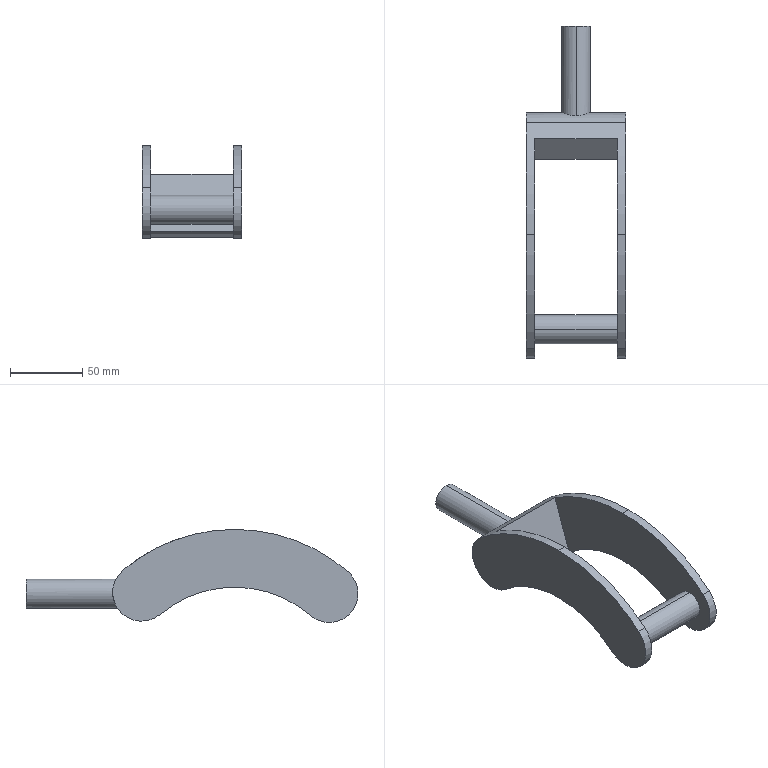Part | SolidWorks | features ICE 4, Extrusion 1 | 1 solid | 20 faces | box 69 x 230 x 64.48 mm | volume 170507 mm3 | cylinder 14 | plane 6 | commonest cylinder face diameters 20 x4 160 x4 40 x3 240 x3
STEP:
#1=CARTESIAN_POINT('',(0.,210.,10.));
#2=VERTEX_POINT('',#1);
#3=CARTESIAN_POINT('',(0.,210.,-10.));
#4=VERTEX_POINT('',#3);
#5=CARTESIAN_POINT('',(0.,210.,0.));
#6=DIRECTION('',(0.,1.,0.));
#7=DIRECTION('',(0.,0.,1.));
#8=AXIS2_PLACEMENT_3D('',#5,#6,#7);
#9=CIRCLE('',#8,10.);
#10=EDGE_CURVE('',#2,#4,#9,.T.);
#11=ORIENTED_EDGE('',*,*,#10,.F.);
#12=CARTESIAN_POINT('',(0.,147.831,10.));
#13=VERTEX_POINT('',#12);
#14=CARTESIAN_POINT('',(0.,210.,10.));
#15=DIRECTION('',(0.,-1.,0.));
#16=VECTOR('',#15,1000.);
#17=LINE('',#14,#16);
#18=EDGE_CURVE('',#2,#13,#17,.T.);
#19=ORIENTED_EDGE('',*,*,#18,.T.);
#20=CARTESIAN_POINT('',(0.,146.742,-10.));
#21=VERTEX_POINT('',#20);
#22=CARTESIAN_POINT('',(0.,147.831,10.));
#23=CARTESIAN_POINT('',(0.6634,147.831,10.));
#24=CARTESIAN_POINT('',(1.339,147.866,9.932));
#25=CARTESIAN_POINT('',(2.636,147.996,9.669));
#26=CARTESIAN_POINT('',(3.265,148.09,9.475));
#27=CARTESIAN_POINT('',(4.486,148.323,8.962));
#28=CARTESIAN_POINT('',(5.059,148.458,8.651));
#29=CARTESIAN_POINT('',(5.866,148.674,8.105));
#30=CARTESIAN_POINT('',(6.126,148.748,7.911));
#31=CARTESIAN_POINT('',(6.63,148.897,7.494));
#32=CARTESIAN_POINT('',(6.871,148.973,7.273));
#33=CARTESIAN_POINT('',(7.557,149.194,6.582));
#34=CARTESIAN_POINT('',(7.966,149.336,6.08));
#35=CARTESIAN_POINT('',(8.509,149.529,5.263));
#36=CARTESIAN_POINT('',(8.679,149.591,4.978));
#37=CARTESIAN_POINT('',(8.988,149.702,4.396));
#38=CARTESIAN_POINT('',(9.128,149.752,4.098));
#39=CARTESIAN_POINT('',(9.501,149.883,3.188));
#40=CARTESIAN_POINT('',(9.691,149.946,2.556));
#41=CARTESIAN_POINT('',(9.882,149.993,1.568));
#42=CARTESIAN_POINT('',(9.929,150.001,1.235));
#43=CARTESIAN_POINT('',(9.989,149.999,0.5732));
#44=CARTESIAN_POINT('',(10.016,149.982,-0.08898));
#45=CARTESIAN_POINT('',(9.977,149.931,-0.7512));
#46=CARTESIAN_POINT('',(9.905,149.864,-1.413));
#47=CARTESIAN_POINT('',(9.852,149.822,-1.744));
#48=CARTESIAN_POINT('',(9.648,149.674,-2.712));
#49=CARTESIAN_POINT('',(9.45,149.548,-3.334));
#50=CARTESIAN_POINT('',(9.065,149.321,-4.234));
#51=CARTESIAN_POINT('',(8.922,149.24,-4.528));
#52=CARTESIAN_POINT('',(8.611,149.07,-5.094));
#53=CARTESIAN_POINT('',(8.444,148.981,-5.367));
#54=CARTESIAN_POINT('',(8.084,148.798,-5.895));
#55=CARTESIAN_POINT('',(7.892,148.703,-6.15));
#56=CARTESIAN_POINT('',(7.483,148.509,-6.641));
#57=CARTESIAN_POINT('',(7.265,148.41,-6.879));
#58=CARTESIAN_POINT('',(6.585,148.113,-7.553));
#59=CARTESIAN_POINT('',(6.094,147.918,-7.954));
#60=CARTESIAN_POINT('',(5.299,147.64,-8.487));
#61=CARTESIAN_POINT('',(5.023,147.55,-8.653));
#62=CARTESIAN_POINT('',(4.452,147.378,-8.96));
#63=CARTESIAN_POINT('',(4.158,147.297,-9.1));
#64=CARTESIAN_POINT('',(3.262,147.076,-9.475));
#65=CARTESIAN_POINT('',(2.642,146.956,-9.667));
#66=CARTESIAN_POINT('',(1.349,146.788,-9.93));
#67=CARTESIAN_POINT('',(0.673,146.742,-10.));
#68=CARTESIAN_POINT('',(0.,146.742,-10.));
#69=B_SPLINE_CURVE_WITH_KNOTS('',3,(#22,#23,#24,#25,#26,#27,#28,#29,#30,#31,#32,#33,#34,#35,#36,#37,#38,#39,#40,#41,#42,#43,#44,#45,#46,#47,#48,#49,#50,#51,#52,#53,#54,#55,#56,#57,#58,#59,#60,#61,#62,#63,#64,#65,#66,#67,#68),.UNSPECIFIED.,.F.,.F.,(4,2,2,2,2,2,2,2,2,2,2,1,2,2,2,2,2,2,2,2,2,2,2,4),(0.03183,0.03381,0.0358,0.03778,0.03878,0.03977,0.04176,0.04275,0.04374,0.04573,0.04672,0.04772,0.04871,0.0497,0.05169,0.05268,0.05367,0.05467,0.05566,0.05765,0.05864,0.05963,0.06162,0.06361),.UNSPECIFIED.);
#70=EDGE_CURVE('',#13,#21,#69,.T.);
#71=ORIENTED_EDGE('',*,*,#70,.T.);
#72=CARTESIAN_POINT('',(0.,210.,-10.));
#73=DIRECTION('',(0.,-1.,0.));
#74=VECTOR('',#73,1000.);
#75=LINE('',#72,#74);
#76=EDGE_CURVE('',#4,#21,#75,.T.);
#77=ORIENTED_EDGE('',*,*,#76,.F.);
#78=EDGE_LOOP('',(#11,#19,#71,#77));
#79=FACE_OUTER_BOUND('',#78,.T.);
#80=CARTESIAN_POINT('',(0.,210.,0.));
#81=DIRECTION('',(0.,-1.,0.));
#82=DIRECTION('',(0.,0.,-1.));
#83=AXIS2_PLACEMENT_3D('',#80,#81,#82);
#84=CYLINDRICAL_SURFACE('',#83,10.);
#85=ADVANCED_FACE('',(#79),#84,.T.);
#86=CARTESIAN_POINT('',(28.5,0.,10.));
#87=VERTEX_POINT('',#86);
#88=CARTESIAN_POINT('',(28.5,0.,-10.));
#89=VERTEX_POINT('',#88);
#90=CARTESIAN_POINT('',(28.5,0.,0.));
#91=DIRECTION('',(-1.,0.,0.));
#92=DIRECTION('',(0.,0.,-1.));
#93=AXIS2_PLACEMENT_3D('',#90,#91,#92);
#94=CIRCLE('',#93,10.);
#95=EDGE_CURVE('',#87,#89,#94,.T.);
#96=ORIENTED_EDGE('',*,*,#95,.T.);
#97=CARTESIAN_POINT('',(-28.5,0.,-10.));
#98=VERTEX_POINT('',#97);
#99=CARTESIAN_POINT('',(29.,0.,-10.));
#100=DIRECTION('',(-1.,0.,0.));
#101=VECTOR('',#100,1000.);
#102=LINE('',#99,#101);
#103=EDGE_CURVE('',#89,#98,#102,.T.);
#104=ORIENTED_EDGE('',*,*,#103,.T.);
#105=CARTESIAN_POINT('',(-28.5,0.,10.));
#106=VERTEX_POINT('',#105);
#107=CARTESIAN_POINT('',(-28.5,0.,0.));
#108=DIRECTION('',(-1.,0.,0.));
#109=DIRECTION('',(0.,0.,-1.));
#110=AXIS2_PLACEMENT_3D('',#107,#108,#109);
#111=CIRCLE('',#110,10.);
#112=EDGE_CURVE('',#106,#98,#111,.T.);
#113=ORIENTED_EDGE('',*,*,#112,.F.);
#114=CARTESIAN_POINT('',(29.,0.,10.));
#115=DIRECTION('',(-1.,0.,0.));
#116=VECTOR('',#115,1000.);
#117=LINE('',#114,#116);
#118=EDGE_CURVE('',#87,#106,#117,.T.);
#119=ORIENTED_EDGE('',*,*,#118,.F.);
#120=EDGE_LOOP('',(#96,#104,#113,#119));
#121=FACE_OUTER_BOUND('',#120,.T.);
#122=CARTESIAN_POINT('',(29.,0.,0.));
#123=DIRECTION('',(-1.,0.,0.));
#124=DIRECTION('',(0.,0.,1.));
#125=AXIS2_PLACEMENT_3D('',#122,#123,#124);
#126=CYLINDRICAL_SURFACE('',#125,10.);
#127=ADVANCED_FACE('',(#121),#126,.T.);
#128=CARTESIAN_POINT('',(-28.5,65.55,4.48));
#129=VERTEX_POINT('',#128);
#130=CARTESIAN_POINT('',(-28.5,117.11,-14.351));
#131=VERTEX_POINT('',#130);
#132=CARTESIAN_POINT('',(-28.5,65.55,-75.52));
#133=DIRECTION('',(-1.,0.,0.));
#134=DIRECTION('',(0.,0.,-1.));
#135=AXIS2_PLACEMENT_3D('',#132,#133,#134);
#136=CIRCLE('',#135,80.);
#137=EDGE_CURVE('',#129,#131,#136,.T.);
#138=ORIENTED_EDGE('',*,*,#137,.F.);
#139=CARTESIAN_POINT('',(-34.5,65.55,4.48));
#140=VERTEX_POINT('',#139);
#141=CARTESIAN_POINT('',(34.5,65.55,4.48));
#142=DIRECTION('',(-1.,0.,0.));
#143=VECTOR('',#142,1000.);
#144=LINE('',#141,#143);
#145=EDGE_CURVE('',#129,#140,#144,.T.);
#146=ORIENTED_EDGE('',*,*,#145,.T.);
#147=CARTESIAN_POINT('',(-34.5,117.11,-14.351));
#148=VERTEX_POINT('',#147);
#149=CARTESIAN_POINT('',(-34.5,65.55,-75.52));
#150=DIRECTION('',(-1.,0.,0.));
#151=DIRECTION('',(0.,0.,-1.));
#152=AXIS2_PLACEMENT_3D('',#149,#150,#151);
#153=CIRCLE('',#152,80.);
#154=EDGE_CURVE('',#140,#148,#153,.T.);
#155=ORIENTED_EDGE('',*,*,#154,.T.);
#156=CARTESIAN_POINT('',(34.5,117.11,-14.351));
#157=DIRECTION('',(-1.,0.,0.));
#158=VECTOR('',#157,1000.);
#159=LINE('',#156,#158);
#160=EDGE_CURVE('',#131,#148,#159,.T.);
#161=ORIENTED_EDGE('',*,*,#160,.F.);
#162=EDGE_LOOP('',(#138,#146,#155,#161));
#163=FACE_OUTER_BOUND('',#162,.T.);
#164=CARTESIAN_POINT('',(34.5,65.55,-75.52));
#165=DIRECTION('',(-1.,0.,0.));
#166=DIRECTION('',(0.,0.,1.));
#167=AXIS2_PLACEMENT_3D('',#164,#165,#166);
#168=CYLINDRICAL_SURFACE('',#167,80.);
#169=ADVANCED_FACE('',(#163),#168,.F.);
#170=CARTESIAN_POINT('',(34.5,65.55,4.48));
#171=VERTEX_POINT('',#170);
#172=CARTESIAN_POINT('',(34.5,117.11,-14.351));
#173=VERTEX_POINT('',#172);
#174=CARTESIAN_POINT('',(34.5,65.55,-75.52));
#175=DIRECTION('',(-1.,0.,0.));
#176=DIRECTION('',(0.,0.,-1.));
#177=AXIS2_PLACEMENT_3D('',#174,#175,#176);
#178=CIRCLE('',#177,80.);
#179=EDGE_CURVE('',#171,#173,#178,.T.);
#180=ORIENTED_EDGE('',*,*,#179,.F.);
#181=CARTESIAN_POINT('',(28.5,65.55,4.48));
#182=VERTEX_POINT('',#181);
#183=CARTESIAN_POINT('',(34.5,65.55,4.48));
#184=DIRECTION('',(-1.,0.,0.));
#185=VECTOR('',#184,1000.);
#186=LINE('',#183,#185);
#187=EDGE_CURVE('',#171,#182,#186,.T.);
#188=ORIENTED_EDGE('',*,*,#187,.T.);
#189=CARTESIAN_POINT('',(28.5,117.11,-14.351));
#190=VERTEX_POINT('',#189);
#191=CARTESIAN_POINT('',(28.5,65.55,-75.52));
#192=DIRECTION('',(-1.,0.,0.));
#193=DIRECTION('',(0.,0.,-1.));
#194=AXIS2_PLACEMENT_3D('',#191,#192,#193);
#195=CIRCLE('',#194,80.);
#196=EDGE_CURVE('',#182,#190,#195,.T.);
#197=ORIENTED_EDGE('',*,*,#196,.T.);
#198=CARTESIAN_POINT('',(34.5,117.11,-14.351));
#199=DIRECTION('',(-1.,0.,0.));
#200=VECTOR('',#199,1000.);
#201=LINE('',#198,#200);
#202=EDGE_CURVE('',#173,#190,#201,.T.);
#203=ORIENTED_EDGE('',*,*,#202,.F.);
#204=EDGE_LOOP('',(#180,#188,#197,#203));
#205=FACE_OUTER_BOUND('',#204,.T.);
#206=CARTESIAN_POINT('',(34.5,65.55,-75.52));
#207=DIRECTION('',(-1.,0.,0.));
#208=DIRECTION('',(0.,0.,1.));
#209=AXIS2_PLACEMENT_3D('',#206,#207,#208);
#210=CYLINDRICAL_SURFACE('',#209,80.);
#211=ADVANCED_FACE('',(#205),#210,.F.);
#212=CARTESIAN_POINT('',(34.5,65.55,44.48));
#213=VERTEX_POINT('',#212);
#214=CARTESIAN_POINT('',(34.5,-13.11,15.104));
#215=VERTEX_POINT('',#214);
#216=CARTESIAN_POINT('',(34.5,65.55,-75.52));
#217=DIRECTION('',(1.,0.,0.));
#218=DIRECTION('',(0.,0.,-1.));
#219=AXIS2_PLACEMENT_3D('',#216,#217,#218);
#220=CIRCLE('',#219,120.);
#221=EDGE_CURVE('',#213,#215,#220,.T.);
#222=ORIENTED_EDGE('',*,*,#221,.F.);
#223=CARTESIAN_POINT('',(28.5,65.55,44.48));
#224=VERTEX_POINT('',#223);
#225=CARTESIAN_POINT('',(34.5,65.55,44.48));
#226=DIRECTION('',(-1.,0.,0.));
#227=VECTOR('',#226,1000.);
#228=LINE('',#225,#227);
#229=EDGE_CURVE('',#213,#224,#228,.T.);
#230=ORIENTED_EDGE('',*,*,#229,.T.);
#231=CARTESIAN_POINT('',(28.5,-13.11,15.104));
#232=VERTEX_POINT('',#231);
#233=CARTESIAN_POINT('',(28.5,65.55,-75.52));
#234=DIRECTION('',(1.,0.,0.));
#235=DIRECTION('',(0.,0.,-1.));
#236=AXIS2_PLACEMENT_3D('',#233,#234,#235);
#237=CIRCLE('',#236,120.);
#238=EDGE_CURVE('',#224,#232,#237,.T.);
#239=ORIENTED_EDGE('',*,*,#238,.T.);
#240=CARTESIAN_POINT('',(34.5,-13.11,15.104));
#241=DIRECTION('',(-1.,0.,0.));
#242=VECTOR('',#241,1000.);
#243=LINE('',#240,#242);
#244=EDGE_CURVE('',#215,#232,#243,.T.);
#245=ORIENTED_EDGE('',*,*,#244,.F.);
#246=EDGE_LOOP('',(#222,#230,#239,#245));
#247=FACE_OUTER_BOUND('',#246,.T.);
#248=CARTESIAN_POINT('',(34.5,65.55,-75.52));
#249=DIRECTION('',(-1.,0.,0.));
#250=DIRECTION('',(0.,0.,1.));
#251=AXIS2_PLACEMENT_3D('',#248,#249,#250);
#252=CYLINDRICAL_SURFACE('',#251,120.);
#253=ADVANCED_FACE('',(#247),#252,.T.);
#254=CARTESIAN_POINT('',(-28.5,65.55,44.48));
#255=VERTEX_POINT('',#254);
#256=CARTESIAN_POINT('',(-28.5,-13.11,15.104));
#257=VERTEX_POINT('',#256);
#258=CARTESIAN_POINT('',(-28.5,65.55,-75.52));
#259=DIRECTION('',(1.,0.,0.));
#260=DIRECTION('',(0.,0.,-1.));
#261=AXIS2_PLACEMENT_3D('',#258,#259,#260);
#262=CIRCLE('',#261,120.);
#263=EDGE_CURVE('',#255,#257,#262,.T.);
#264=ORIENTED_EDGE('',*,*,#263,.F.);
#265=CARTESIAN_POINT('',(-34.5,65.55,44.48));
#266=VERTEX_POINT('',#265);
#267=CARTESIAN_POINT('',(34.5,65.55,44.48));
#268=DIRECTION('',(-1.,0.,0.));
#269=VECTOR('',#268,1000.);
#270=LINE('',#267,#269);
#271=EDGE_CURVE('',#255,#266,#270,.T.);
#272=ORIENTED_EDGE('',*,*,#271,.T.);
#273=CARTESIAN_POINT('',(-34.5,-13.11,15.104));
#274=VERTEX_POINT('',#273);
#275=CARTESIAN_POINT('',(-34.5,65.55,-75.52));
#276=DIRECTION('',(1.,0.,0.));
#277=DIRECTION('',(0.,0.,-1.));
#278=AXIS2_PLACEMENT_3D('',#275,#276,#277);
#279=CIRCLE('',#278,120.);
#280=EDGE_CURVE('',#266,#274,#279,.T.);
#281=ORIENTED_EDGE('',*,*,#280,.T.);
#282=CARTESIAN_POINT('',(34.5,-13.11,15.104));
#283=DIRECTION('',(-1.,0.,0.));
#284=VECTOR('',#283,1000.);
#285=LINE('',#282,#284);
#286=EDGE_CURVE('',#257,#274,#285,.T.);
#287=ORIENTED_EDGE('',*,*,#286,.F.);
#288=EDGE_LOOP('',(#264,#272,#281,#287));
#289=FACE_OUTER_BOUND('',#288,.T.);
#290=CARTESIAN_POINT('',(34.5,65.55,-75.52));
#291=DIRECTION('',(-1.,0.,0.));
#292=DIRECTION('',(0.,0.,1.));
#293=AXIS2_PLACEMENT_3D('',#290,#291,#292);
#294=CYLINDRICAL_SURFACE('',#293,120.);
#295=ADVANCED_FACE('',(#289),#294,.T.);
#296=CARTESIAN_POINT('',(28.5,117.742,-14.862));
#297=VERTEX_POINT('',#296);
#298=CARTESIAN_POINT('',(28.5,130.,0.9408));
#299=DIRECTION('',(-1.,0.,0.));
#300=DIRECTION('',(0.,0.,1.));
#301=AXIS2_PLACEMENT_3D('',#298,#299,#300);
#302=CIRCLE('',#301,20.);
#303=EDGE_CURVE('',#297,#190,#302,.T.);
#304=ORIENTED_EDGE('',*,*,#303,.F.);
#305=CARTESIAN_POINT('',(-28.5,117.742,-14.862));
#306=VERTEX_POINT('',#305);
#307=CARTESIAN_POINT('',(34.5,117.742,-14.862));
#308=DIRECTION('',(1.,0.,0.));
#309=VECTOR('',#308,1000.);
#310=LINE('',#307,#309);
#311=EDGE_CURVE('',#306,#297,#310,.T.);
#312=ORIENTED_EDGE('',*,*,#311,.F.);
#313=CARTESIAN_POINT('',(-28.5,130.,0.9408));
#314=DIRECTION('',(1.,0.,0.));
#315=DIRECTION('',(0.,0.,-1.));
#316=AXIS2_PLACEMENT_3D('',#313,#314,#315);
#317=CIRCLE('',#316,20.);
#318=EDGE_CURVE('',#131,#306,#317,.T.);
#319=ORIENTED_EDGE('',*,*,#318,.F.);
#320=ORIENTED_EDGE('',*,*,#160,.T.);
#321=CARTESIAN_POINT('',(-34.5,142.89,16.233));
#322=VERTEX_POINT('',#321);
#323=CARTESIAN_POINT('',(-34.5,130.,0.9408));
#324=DIRECTION('',(1.,0.,0.));
#325=DIRECTION('',(0.,0.,-1.));
#326=AXIS2_PLACEMENT_3D('',#323,#324,#325);
#327=CIRCLE('',#326,20.);
#328=EDGE_CURVE('',#148,#322,#327,.T.);
#329=ORIENTED_EDGE('',*,*,#328,.T.);
#330=CARTESIAN_POINT('',(34.5,142.89,16.233));
#331=VERTEX_POINT('',#330);
#332=CARTESIAN_POINT('',(34.5,142.89,16.233));
#333=DIRECTION('',(-1.,0.,0.));
#334=VECTOR('',#333,1000.);
#335=LINE('',#332,#334);
#336=EDGE_CURVE('',#331,#322,#335,.T.);
#337=ORIENTED_EDGE('',*,*,#336,.F.);
#338=CARTESIAN_POINT('',(34.5,130.,0.9408));
#339=DIRECTION('',(1.,0.,0.));
#340=DIRECTION('',(0.,0.,-1.));
#341=AXIS2_PLACEMENT_3D('',#338,#339,#340);
#342=CIRCLE('',#341,20.);
#343=EDGE_CURVE('',#173,#331,#342,.T.);
#344=ORIENTED_EDGE('',*,*,#343,.F.);
#345=ORIENTED_EDGE('',*,*,#202,.T.);
#346=EDGE_LOOP('',(#304,#312,#319,#320,#329,#337,#344,#345));
#347=FACE_OUTER_BOUND('',#346,.T.);
#348=CARTESIAN_POINT('',(0.,146.742,-10.));
#349=CARTESIAN_POINT('',(-0.674,146.742,-10.));
#350=CARTESIAN_POINT('',(-1.333,146.787,-9.933));
#351=CARTESIAN_POINT('',(-2.625,146.953,-9.672));
#352=CARTESIAN_POINT('',(-3.263,147.076,-9.475));
#353=CARTESIAN_POINT('',(-4.461,147.372,-8.973));
#354=CARTESIAN_POINT('',(-5.027,147.545,-8.669));
#355=CARTESIAN_POINT('',(-6.098,147.919,-7.951));
#356=CARTESIAN_POINT('',(-6.592,148.117,-7.546));
#357=CARTESIAN_POINT('',(-7.268,148.411,-6.876));
#358=CARTESIAN_POINT('',(-7.483,148.509,-6.641));
#359=CARTESIAN_POINT('',(-7.892,148.703,-6.149));
#360=CARTESIAN_POINT('',(-8.087,148.799,-5.891));
#361=CARTESIAN_POINT('',(-8.628,149.076,-5.095));
#362=CARTESIAN_POINT('',(-8.936,149.246,-4.534));
#363=CARTESIAN_POINT('',(-9.318,149.47,-3.644));
#364=CARTESIAN_POINT('',(-9.432,149.54,-3.338));
#365=CARTESIAN_POINT('',(-9.631,149.667,-2.71));
#366=CARTESIAN_POINT('',(-9.716,149.723,-2.39));
#367=CARTESIAN_POINT('',(-9.92,149.87,-1.424));
#368=CARTESIAN_POINT('',(-9.992,149.938,-0.7701));
#369=CARTESIAN_POINT('',(-10.003,149.99,0.2283));
#370=CARTESIAN_POINT('',(-9.99,149.999,0.5662));
#371=CARTESIAN_POINT('',(-9.929,150.001,1.233));
#372=CARTESIAN_POINT('',(-9.883,149.993,1.563));
#373=CARTESIAN_POINT('',(-9.757,149.962,2.214));
#374=CARTESIAN_POINT('',(-9.679,149.939,2.536));
#375=CARTESIAN_POINT('',(-9.489,149.878,3.173));
#376=CARTESIAN_POINT('',(-9.378,149.839,3.489));
#377=CARTESIAN_POINT('',(-8.999,149.706,4.411));
#378=CARTESIAN_POINT('',(-8.691,149.594,4.99));
#379=CARTESIAN_POINT('',(-8.147,149.401,5.808));
#380=CARTESIAN_POINT('',(-7.951,149.332,6.073));
#381=CARTESIAN_POINT('',(-7.537,149.19,6.581));
#382=CARTESIAN_POINT('',(-7.319,149.117,6.822));
#383=CARTESIAN_POINT('',(-6.633,148.896,7.512));
#384=CARTESIAN_POINT('',(-6.133,148.745,7.925));
#385=CARTESIAN_POINT('',(-5.045,148.455,8.659));
#386=CARTESIAN_POINT('',(-4.47,148.32,8.969));
#387=CARTESIAN_POINT('',(-3.567,148.148,9.348));
#388=CARTESIAN_POINT('',(-3.259,148.095,9.46));
#389=CARTESIAN_POINT('',(-2.628,148.002,9.654));
#390=CARTESIAN_POINT('',(-2.303,147.962,9.737));
#391=CARTESIAN_POINT('',(-1.323,147.864,9.934));
#392=CARTESIAN_POINT('',(-0.6644,147.831,10.));
#393=CARTESIAN_POINT('',(0.,147.831,10.));
#394=B_SPLINE_CURVE_WITH_KNOTS('',3,(#348,#349,#350,#351,#352,#353,#354,#355,#356,#357,#358,#359,#360,#361,#362,#363,#364,#365,#366,#367,#368,#369,#370,#371,#372,#373,#374,#375,#376,#377,#378,#379,#380,#381,#382,#383,#384,#385,#386,#387,#388,#389,#390,#391,#392,#393),.UNSPECIFIED.,.F.,.F.,(4,2,2,2,2,2,2,2,2,2,2,2,2,2,2,2,2,2,2,2,2,2,4),(0.,0.001989,0.003978,0.005967,0.007956,0.008951,0.009946,0.01193,0.01293,0.01392,0.01591,0.01691,0.0179,0.0189,0.01989,0.02188,0.02287,0.02387,0.02586,0.02785,0.02884,0.02984,0.03183),.UNSPECIFIED.);
#395=EDGE_CURVE('',#21,#13,#394,.T.);
#396=ORIENTED_EDGE('',*,*,#395,.F.);
#397=ORIENTED_EDGE('',*,*,#70,.F.);
#398=EDGE_LOOP('',(#396,#397));
#399=FACE_BOUND('',#398,.T.);
#400=CARTESIAN_POINT('',(34.5,130.,0.9408));
#401=DIRECTION('',(-1.,0.,0.));
#402=DIRECTION('',(0.,0.,1.));
#403=AXIS2_PLACEMENT_3D('',#400,#401,#402);
#404=CYLINDRICAL_SURFACE('',#403,20.);
#405=ADVANCED_FACE('',(#347,#399),#404,.T.);
#406=ORIENTED_EDGE('',*,*,#229,.F.);
#407=CARTESIAN_POINT('',(34.5,65.55,-75.52));
#408=DIRECTION('',(1.,0.,0.));
#409=DIRECTION('',(0.,0.,-1.));
#410=AXIS2_PLACEMENT_3D('',#407,#408,#409);
#411=CIRCLE('',#410,120.);
#412=EDGE_CURVE('',#331,#213,#411,.T.);
#413=ORIENTED_EDGE('',*,*,#412,.F.);
#414=ORIENTED_EDGE('',*,*,#336,.T.);
#415=CARTESIAN_POINT('',(-34.5,65.55,-75.52));
#416=DIRECTION('',(1.,0.,0.));
#417=DIRECTION('',(0.,0.,-1.));
#418=AXIS2_PLACEMENT_3D('',#415,#416,#417);
#419=CIRCLE('',#418,120.);
#420=EDGE_CURVE('',#322,#266,#419,.T.);
#421=ORIENTED_EDGE('',*,*,#420,.T.);
#422=ORIENTED_EDGE('',*,*,#271,.F.);
#423=CARTESIAN_POINT('',(-28.5,131.974,24.42));
#424=VERTEX_POINT('',#423);
#425=CARTESIAN_POINT('',(-28.5,65.55,-75.52));
#426=DIRECTION('',(1.,0.,0.));
#427=DIRECTION('',(0.,0.,-1.));
#428=AXIS2_PLACEMENT_3D('',#425,#426,#427);
#429=CIRCLE('',#428,120.);
#430=EDGE_CURVE('',#424,#255,#429,.T.);
#431=ORIENTED_EDGE('',*,*,#430,.F.);
#432=CARTESIAN_POINT('',(28.5,131.974,24.42));
#433=VERTEX_POINT('',#432);
#434=CARTESIAN_POINT('',(34.5,131.974,24.42));
#435=DIRECTION('',(-1.,0.,0.));
#436=VECTOR('',#435,1000.);
#437=LINE('',#434,#436);
#438=EDGE_CURVE('',#433,#424,#437,.T.);
#439=ORIENTED_EDGE('',*,*,#438,.F.);
#440=CARTESIAN_POINT('',(28.5,65.55,-75.52));
#441=DIRECTION('',(1.,0.,0.));
#442=DIRECTION('',(0.,0.,-1.));
#443=AXIS2_PLACEMENT_3D('',#440,#441,#442);
#444=CIRCLE('',#443,120.);
#445=EDGE_CURVE('',#433,#224,#444,.T.);
#446=ORIENTED_EDGE('',*,*,#445,.T.);
#447=EDGE_LOOP('',(#406,#413,#414,#421,#422,#431,#439,#446));
#448=FACE_OUTER_BOUND('',#447,.T.);
#449=CARTESIAN_POINT('',(34.5,65.55,-75.52));
#450=DIRECTION('',(-1.,0.,0.));
#451=DIRECTION('',(0.,0.,1.));
#452=AXIS2_PLACEMENT_3D('',#449,#450,#451);
#453=CYLINDRICAL_SURFACE('',#452,120.);
#454=ADVANCED_FACE('',(#448),#453,.T.);
#455=ORIENTED_EDGE('',*,*,#187,.F.);
#456=CARTESIAN_POINT('',(34.5,13.11,-15.104));
#457=VERTEX_POINT('',#456);
#458=CARTESIAN_POINT('',(34.5,65.55,-75.52));
#459=DIRECTION('',(-1.,0.,0.));
#460=DIRECTION('',(0.,0.,-1.));
#461=AXIS2_PLACEMENT_3D('',#458,#459,#460);
#462=CIRCLE('',#461,80.);
#463=EDGE_CURVE('',#457,#171,#462,.T.);
#464=ORIENTED_EDGE('',*,*,#463,.F.);
#465=CARTESIAN_POINT('',(28.5,13.11,-15.104));
#466=VERTEX_POINT('',#465);
#467=CARTESIAN_POINT('',(34.5,13.11,-15.104));
#468=DIRECTION('',(-1.,0.,0.));
#469=VECTOR('',#468,1000.);
#470=LINE('',#467,#469);
#471=EDGE_CURVE('',#457,#466,#470,.T.);
#472=ORIENTED_EDGE('',*,*,#471,.T.);
#473=CARTESIAN_POINT('',(28.5,65.55,-75.52));
#474=DIRECTION('',(-1.,0.,0.));
#475=DIRECTION('',(0.,0.,-1.));
#476=AXIS2_PLACEMENT_3D('',#473,#474,#475);
#477=CIRCLE('',#476,80.);
#478=EDGE_CURVE('',#466,#182,#477,.T.);
#479=ORIENTED_EDGE('',*,*,#478,.T.);
#480=EDGE_LOOP('',(#455,#464,#472,#479));
#481=FACE_OUTER_BOUND('',#480,.T.);
#482=CARTESIAN_POINT('',(34.5,65.55,-75.52));
#483=DIRECTION('',(-1.,0.,0.));
#484=DIRECTION('',(0.,0.,1.));
#485=AXIS2_PLACEMENT_3D('',#482,#483,#484);
#486=CYLINDRICAL_SURFACE('',#485,80.);
#487=ADVANCED_FACE('',(#481),#486,.F.);
#488=ORIENTED_EDGE('',*,*,#145,.F.);
#489=CARTESIAN_POINT('',(-28.5,13.11,-15.104));
#490=VERTEX_POINT('',#489);
#491=CARTESIAN_POINT('',(-28.5,65.55,-75.52));
#492=DIRECTION('',(-1.,0.,0.));
#493=DIRECTION('',(0.,0.,-1.));
#494=AXIS2_PLACEMENT_3D('',#491,#492,#493);
#495=CIRCLE('',#494,80.);
#496=EDGE_CURVE('',#490,#129,#495,.T.);
#497=ORIENTED_EDGE('',*,*,#496,.F.);
#498=CARTESIAN_POINT('',(-34.5,13.11,-15.104));
#499=VERTEX_POINT('',#498);
#500=CARTESIAN_POINT('',(34.5,13.11,-15.104));
#501=DIRECTION('',(-1.,0.,0.));
#502=VECTOR('',#501,1000.);
#503=LINE('',#500,#502);
#504=EDGE_CURVE('',#490,#499,#503,.T.);
#505=ORIENTED_EDGE('',*,*,#504,.T.);
#506=CARTESIAN_POINT('',(-34.5,65.55,-75.52));
#507=DIRECTION('',(-1.,0.,0.));
#508=DIRECTION('',(0.,0.,-1.));
#509=AXIS2_PLACEMENT_3D('',#506,#507,#508);
#510=CIRCLE('',#509,80.);
#511=EDGE_CURVE('',#499,#140,#510,.T.);
#512=ORIENTED_EDGE('',*,*,#511,.T.);
#513=EDGE_LOOP('',(#488,#497,#505,#512));
#514=FACE_OUTER_BOUND('',#513,.T.);
#515=CARTESIAN_POINT('',(34.5,65.55,-75.52));
#516=DIRECTION('',(-1.,0.,0.));
#517=DIRECTION('',(0.,0.,1.));
#518=AXIS2_PLACEMENT_3D('',#515,#516,#517);
#519=CYLINDRICAL_SURFACE('',#518,80.);
#520=ADVANCED_FACE('',(#514),#519,.F.);
#521=CARTESIAN_POINT('',(-28.5,0.,0.));
#522=DIRECTION('',(1.,0.,0.));
#523=DIRECTION('',(0.,0.,-1.));
#524=AXIS2_PLACEMENT_3D('',#521,#522,#523);
#525=CIRCLE('',#524,20.);
#526=EDGE_CURVE('',#257,#490,#525,.T.);
#527=ORIENTED_EDGE('',*,*,#526,.F.);
#528=ORIENTED_EDGE('',*,*,#286,.T.);
#529=CARTESIAN_POINT('',(-34.5,0.,0.));
#530=DIRECTION('',(1.,0.,0.));
#531=DIRECTION('',(0.,0.,-1.));
#532=AXIS2_PLACEMENT_3D('',#529,#530,#531);
#533=CIRCLE('',#532,20.);
#534=EDGE_CURVE('',#274,#499,#533,.T.);
#535=ORIENTED_EDGE('',*,*,#534,.T.);
#536=ORIENTED_EDGE('',*,*,#504,.F.);
#537=EDGE_LOOP('',(#527,#528,#535,#536));
#538=FACE_OUTER_BOUND('',#537,.T.);
#539=CARTESIAN_POINT('',(34.5,0.,0.));
#540=DIRECTION('',(-1.,0.,0.));
#541=DIRECTION('',(0.,0.,1.));
#542=AXIS2_PLACEMENT_3D('',#539,#540,#541);
#543=CYLINDRICAL_SURFACE('',#542,20.);
#544=ADVANCED_FACE('',(#538),#543,.T.);
#545=ORIENTED_EDGE('',*,*,#244,.T.);
#546=CARTESIAN_POINT('',(28.5,0.,0.));
#547=DIRECTION('',(1.,0.,0.));
#548=DIRECTION('',(0.,0.,-1.));
#549=AXIS2_PLACEMENT_3D('',#546,#547,#548);
#550=CIRCLE('',#549,20.);
#551=EDGE_CURVE('',#232,#466,#550,.T.);
#552=ORIENTED_EDGE('',*,*,#551,.T.);
#553=ORIENTED_EDGE('',*,*,#471,.F.);
#554=CARTESIAN_POINT('',(34.5,0.,0.));
#555=DIRECTION('',(1.,0.,0.));
#556=DIRECTION('',(0.,0.,-1.));
#557=AXIS2_PLACEMENT_3D('',#554,#555,#556);
#558=CIRCLE('',#557,20.);
#559=EDGE_CURVE('',#215,#457,#558,.T.);
#560=ORIENTED_EDGE('',*,*,#559,.F.);
#561=EDGE_LOOP('',(#545,#552,#553,#560));
#562=FACE_OUTER_BOUND('',#561,.T.);
#563=CARTESIAN_POINT('',(34.5,0.,0.));
#564=DIRECTION('',(-1.,0.,0.));
#565=DIRECTION('',(0.,0.,1.));
#566=AXIS2_PLACEMENT_3D('',#563,#564,#565);
#567=CYLINDRICAL_SURFACE('',#566,20.);
#568=ADVANCED_FACE('',(#562),#567,.T.);
#569=ORIENTED_EDGE('',*,*,#343,.T.);
#570=ORIENTED_EDGE('',*,*,#412,.T.);
#571=ORIENTED_EDGE('',*,*,#221,.T.);
#572=ORIENTED_EDGE('',*,*,#559,.T.);
#573=ORIENTED_EDGE('',*,*,#463,.T.);
#574=ORIENTED_EDGE('',*,*,#179,.T.);
#575=EDGE_LOOP('',(#569,#570,#571,#572,#573,#574));
#576=FACE_OUTER_BOUND('',#575,.T.);
#577=CARTESIAN_POINT('',(34.5,97.775,-37.289));
#578=DIRECTION('',(1.,0.,0.));
#579=DIRECTION('',(0.,0.,-1.));
#580=AXIS2_PLACEMENT_3D('',#577,#578,#579);
#581=PLANE('',#580);
#582=ADVANCED_FACE('',(#576),#581,.T.);
#583=ORIENTED_EDGE('',*,*,#328,.F.);
#584=ORIENTED_EDGE('',*,*,#154,.F.);
#585=ORIENTED_EDGE('',*,*,#511,.F.);
#586=ORIENTED_EDGE('',*,*,#534,.F.);
#587=ORIENTED_EDGE('',*,*,#280,.F.);
#588=ORIENTED_EDGE('',*,*,#420,.F.);
#589=EDGE_LOOP('',(#583,#584,#585,#586,#587,#588));
#590=FACE_OUTER_BOUND('',#589,.T.);
#591=CARTESIAN_POINT('',(-34.5,97.775,-37.289));
#592=DIRECTION('',(1.,0.,0.));
#593=DIRECTION('',(0.,0.,-1.));
#594=AXIS2_PLACEMENT_3D('',#591,#592,#593);
#595=PLANE('',#594);
#596=ADVANCED_FACE('',(#590),#595,.F.);
#597=ORIENTED_EDGE('',*,*,#112,.T.);
#598=CARTESIAN_POINT('',(-28.5,0.,0.));
#599=DIRECTION('',(-1.,0.,0.));
#600=DIRECTION('',(0.,0.,-1.));
#601=AXIS2_PLACEMENT_3D('',#598,#599,#600);
#602=CIRCLE('',#601,10.);
#603=EDGE_CURVE('',#98,#106,#602,.T.);
#604=ORIENTED_EDGE('',*,*,#603,.T.);
#605=EDGE_LOOP('',(#597,#604));
#606=FACE_BOUND('',#605,.T.);
#607=ORIENTED_EDGE('',*,*,#430,.T.);
#608=ORIENTED_EDGE('',*,*,#263,.T.);
#609=ORIENTED_EDGE('',*,*,#526,.T.);
#610=ORIENTED_EDGE('',*,*,#496,.T.);
#611=ORIENTED_EDGE('',*,*,#137,.T.);
#612=ORIENTED_EDGE('',*,*,#318,.T.);
#613=CARTESIAN_POINT('',(-28.5,111.748,-31.404));
#614=DIRECTION('',(0.,0.3406,0.9402));
#615=VECTOR('',#614,1000.);
#616=LINE('',#613,#615);
#617=EDGE_CURVE('',#306,#424,#616,.T.);
#618=ORIENTED_EDGE('',*,*,#617,.T.);
#619=EDGE_LOOP('',(#607,#608,#609,#610,#611,#612,#618));
#620=FACE_OUTER_BOUND('',#619,.T.);
#621=CARTESIAN_POINT('',(-28.5,0.,0.));
#622=DIRECTION('',(1.,0.,0.));
#623=DIRECTION('',(0.,0.,-1.));
#624=AXIS2_PLACEMENT_3D('',#621,#622,#623);
#625=PLANE('',#624);
#626=ADVANCED_FACE('',(#606,#620),#625,.T.);
#627=ORIENTED_EDGE('',*,*,#95,.F.);
#628=CARTESIAN_POINT('',(28.5,0.,0.));
#629=DIRECTION('',(-1.,0.,0.));
#630=DIRECTION('',(0.,0.,-1.));
#631=AXIS2_PLACEMENT_3D('',#628,#629,#630);
#632=CIRCLE('',#631,10.);
#633=EDGE_CURVE('',#89,#87,#632,.T.);
#634=ORIENTED_EDGE('',*,*,#633,.F.);
#635=EDGE_LOOP('',(#627,#634));
#636=FACE_BOUND('',#635,.T.);
#637=ORIENTED_EDGE('',*,*,#303,.T.);
#638=ORIENTED_EDGE('',*,*,#196,.F.);
#639=ORIENTED_EDGE('',*,*,#478,.F.);
#640=ORIENTED_EDGE('',*,*,#551,.F.);
#641=ORIENTED_EDGE('',*,*,#238,.F.);
#642=ORIENTED_EDGE('',*,*,#445,.F.);
#643=CARTESIAN_POINT('',(28.5,111.748,-31.404));
#644=DIRECTION('',(0.,-0.3406,-0.9402));
#645=VECTOR('',#644,1000.);
#646=LINE('',#643,#645);
#647=EDGE_CURVE('',#433,#297,#646,.T.);
#648=ORIENTED_EDGE('',*,*,#647,.T.);
#649=EDGE_LOOP('',(#637,#638,#639,#640,#641,#642,#648));
#650=FACE_OUTER_BOUND('',#649,.T.);
#651=CARTESIAN_POINT('',(28.5,0.,0.));
#652=DIRECTION('',(1.,0.,0.));
#653=DIRECTION('',(0.,0.,-1.));
#654=AXIS2_PLACEMENT_3D('',#651,#652,#653);
#655=PLANE('',#654);
#656=ADVANCED_FACE('',(#636,#650),#655,.F.);
#657=ORIENTED_EDGE('',*,*,#438,.T.);
#658=ORIENTED_EDGE('',*,*,#617,.F.);
#659=ORIENTED_EDGE('',*,*,#311,.T.);
#660=ORIENTED_EDGE('',*,*,#647,.F.);
#661=EDGE_LOOP('',(#657,#658,#659,#660));
#662=FACE_OUTER_BOUND('',#661,.T.);
#663=CARTESIAN_POINT('',(-170.08,111.748,-31.404));
#664=DIRECTION('',(0.,-0.9402,0.3406));
#665=DIRECTION('',(0.,-0.3406,-0.9402));
#666=AXIS2_PLACEMENT_3D('',#663,#664,#665);
#667=PLANE('',#666);
#668=ADVANCED_FACE('',(#662),#667,.T.);
#669=ORIENTED_EDGE('',*,*,#103,.F.);
#670=ORIENTED_EDGE('',*,*,#633,.T.);
#671=ORIENTED_EDGE('',*,*,#118,.T.);
#672=ORIENTED_EDGE('',*,*,#603,.F.);
#673=EDGE_LOOP('',(#669,#670,#671,#672));
#674=FACE_OUTER_BOUND('',#673,.T.);
#675=CARTESIAN_POINT('',(29.,0.,0.));
#676=DIRECTION('',(-1.,0.,0.));
#677=DIRECTION('',(0.,0.,1.));
#678=AXIS2_PLACEMENT_3D('',#675,#676,#677);
#679=CYLINDRICAL_SURFACE('',#678,10.);
#680=ADVANCED_FACE('',(#674),#679,.T.);
#681=ORIENTED_EDGE('',*,*,#18,.F.);
#682=CARTESIAN_POINT('',(0.,210.,0.));
#683=DIRECTION('',(0.,1.,0.));
#684=DIRECTION('',(0.,0.,1.));
#685=AXIS2_PLACEMENT_3D('',#682,#683,#684);
#686=CIRCLE('',#685,10.);
#687=EDGE_CURVE('',#4,#2,#686,.T.);
#688=ORIENTED_EDGE('',*,*,#687,.F.);
#689=ORIENTED_EDGE('',*,*,#76,.T.);
#690=ORIENTED_EDGE('',*,*,#395,.T.);
#691=EDGE_LOOP('',(#681,#688,#689,#690));
#692=FACE_OUTER_BOUND('',#691,.T.);
#693=CARTESIAN_POINT('',(0.,210.,0.));
#694=DIRECTION('',(0.,-1.,0.));
#695=DIRECTION('',(0.,0.,-1.));
#696=AXIS2_PLACEMENT_3D('',#693,#694,#695);
#697=CYLINDRICAL_SURFACE('',#696,10.);
#698=ADVANCED_FACE('',(#692),#697,.T.);
#699=ORIENTED_EDGE('',*,*,#687,.T.);
#700=ORIENTED_EDGE('',*,*,#10,.T.);
#701=EDGE_LOOP('',(#699,#700));
#702=FACE_OUTER_BOUND('',#701,.T.);
#703=CARTESIAN_POINT('',(0.,210.,0.));
#704=DIRECTION('',(0.,1.,0.));
#705=DIRECTION('',(0.,0.,1.));
#706=AXIS2_PLACEMENT_3D('',#703,#704,#705);
#707=PLANE('',#706);
#708=ADVANCED_FACE('',(#702),#707,.T.);
#709=CLOSED_SHELL('',(#85,#127,#169,#211,#253,#295,#405,#454,#487,#520,#544,#568,#582,#596,#626,#656,#668,#680,#698,#708));
#710=MANIFOLD_SOLID_BREP('',#709);
#711=CARTESIAN_POINT('',(0.,0.,0.));
#712=DIRECTION('',(0.,0.,1.));
#713=DIRECTION('',(1.,0.,0.));
#714=AXIS2_PLACEMENT_3D('',#711,#712,#713);
#715=(LENGTH_UNIT()NAMED_UNIT(*)SI_UNIT(.MILLI.,.METRE.));
#716=UNCERTAINTY_MEASURE_WITH_UNIT(LENGTH_MEASURE(0.00001),#715,'','');
#717=(NAMED_UNIT(*)PLANE_ANGLE_UNIT()SI_UNIT($,.RADIAN.));
#718=(NAMED_UNIT(*)SI_UNIT($,.STERADIAN.)SOLID_ANGLE_UNIT());
#719=(GEOMETRIC_REPRESENTATION_CONTEXT(3)GLOBAL_UNCERTAINTY_ASSIGNED_CONTEXT((#716))GLOBAL_UNIT_ASSIGNED_CONTEXT((#715,#717,#718))REPRESENTATION_CONTEXT('',''));
#720=ADVANCED_BREP_SHAPE_REPRESENTATION('',(#710,#714),#719);